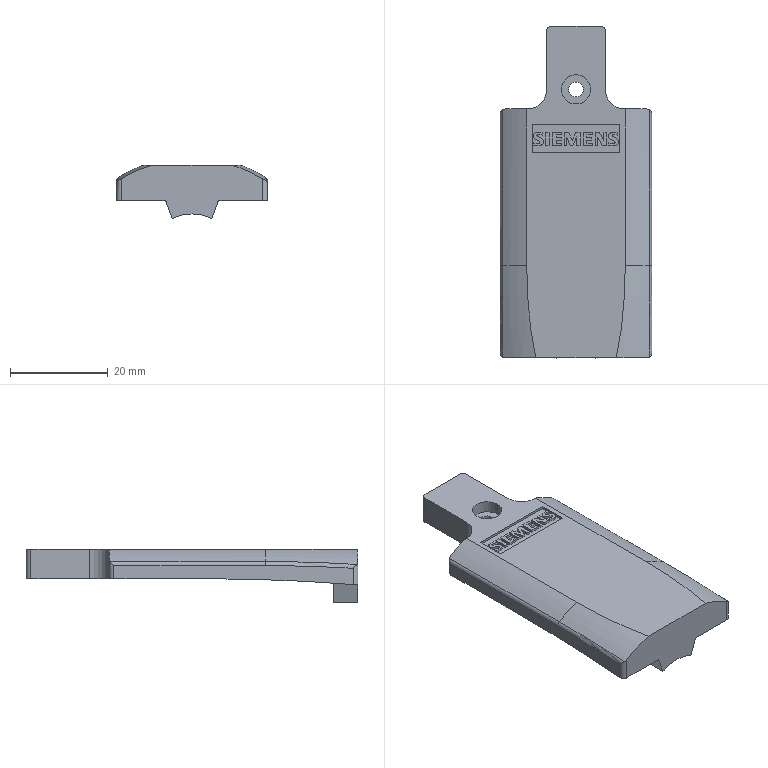Part | STEP file | 2023_07_21_12_39_19_0141 | 1 solid | 139 faces | box 31 x 68 x 10.875 mm | volume 10432 mm3 | plane 83 | cylinder 52 | torus 4 | commonest cylinder face diameters 2 x8 0.315 x2 0.394 x2 0.453 x2 0.627 x2 1.418 x2